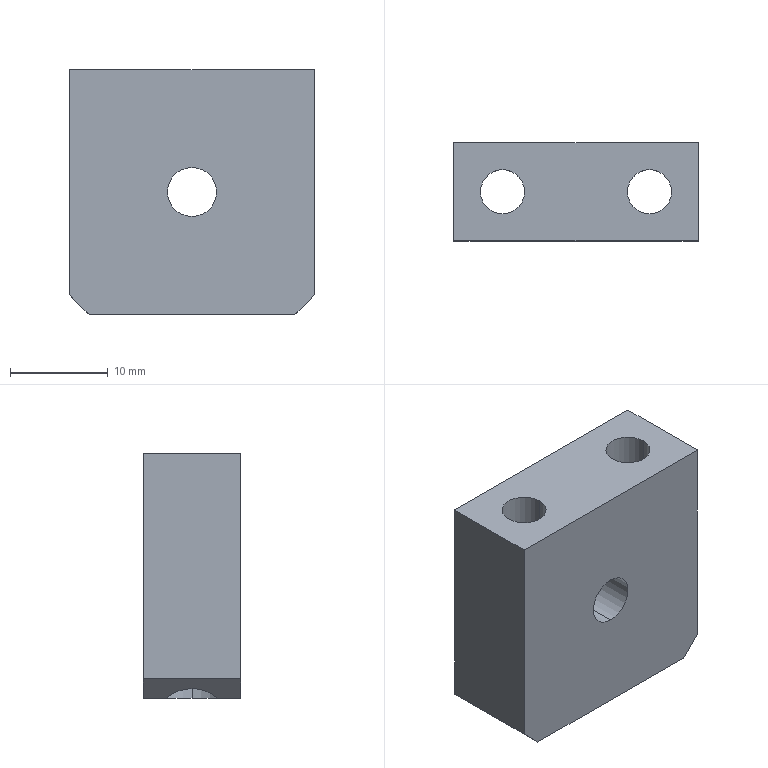Part | SolidWorks | features HoleWzd 2, Chamfer 1, Extrusion 1 | 1 solid | 20 faces | box 25 x 10 x 25 mm | volume 3874 mm3 | cylinder 10 | plane 10 | commonest cylinder face diameters 4.5 x4 8 x4 5 x2
STEP:
#1=CARTESIAN_POINT('',(11.5,5.,7.1));
#2=VERTEX_POINT('',#1);
#3=CARTESIAN_POINT('',(3.5,5.,7.1));
#4=VERTEX_POINT('',#3);
#5=CARTESIAN_POINT('',(7.5,5.,7.1));
#6=DIRECTION('',(0.,0.,-1.));
#7=DIRECTION('',(-1.,0.,0.));
#8=AXIS2_PLACEMENT_3D('',#5,#6,#7);
#9=CIRCLE('',#8,4.);
#10=EDGE_CURVE('',#2,#4,#9,.T.);
#11=ORIENTED_EDGE('',*,*,#10,.F.);
#12=CARTESIAN_POINT('',(11.5,5.,-11.5));
#13=VERTEX_POINT('',#12);
#14=CARTESIAN_POINT('',(11.5,5.,-12.5));
#15=DIRECTION('',(0.,0.,-1.));
#16=VECTOR('',#15,1000.);
#17=LINE('',#14,#16);
#18=EDGE_CURVE('',#2,#13,#17,.T.);
#19=ORIENTED_EDGE('',*,*,#18,.T.);
#20=CARTESIAN_POINT('',(10.5,2.354,-12.5));
#21=VERTEX_POINT('',#20);
#22=CARTESIAN_POINT('',(11.5,5.,-11.5));
#23=CARTESIAN_POINT('',(11.5,4.015,-11.5));
#24=CARTESIAN_POINT('',(11.152,3.093,-11.848));
#25=CARTESIAN_POINT('',(10.5,2.354,-12.5));
#26=(BOUNDED_CURVE()B_SPLINE_CURVE(3,(#22,#23,#24,#25),.UNSPECIFIED.,.F.,.F.)B_SPLINE_CURVE_WITH_KNOTS((4,4),(3.142,3.864),.UNSPECIFIED.)CURVE()GEOMETRIC_REPRESENTATION_ITEM()RATIONAL_B_SPLINE_CURVE((1.,0.9569,0.9569,1.))REPRESENTATION_ITEM(''));
#27=EDGE_CURVE('',#13,#21,#26,.T.);
#28=ORIENTED_EDGE('',*,*,#27,.T.);
#29=CARTESIAN_POINT('',(3.5,5.,-12.5));
#30=VERTEX_POINT('',#29);
#31=CARTESIAN_POINT('',(7.5,5.,-12.5));
#32=DIRECTION('',(0.,0.,-1.));
#33=DIRECTION('',(-1.,0.,0.));
#34=AXIS2_PLACEMENT_3D('',#31,#32,#33);
#35=CIRCLE('',#34,4.);
#36=EDGE_CURVE('',#21,#30,#35,.T.);
#37=ORIENTED_EDGE('',*,*,#36,.T.);
#38=CARTESIAN_POINT('',(3.5,5.,-12.5));
#39=DIRECTION('',(0.,0.,-1.));
#40=VECTOR('',#39,1000.);
#41=LINE('',#38,#40);
#42=EDGE_CURVE('',#4,#30,#41,.T.);
#43=ORIENTED_EDGE('',*,*,#42,.F.);
#44=EDGE_LOOP('',(#11,#19,#28,#37,#43));
#45=FACE_OUTER_BOUND('',#44,.T.);
#46=CARTESIAN_POINT('',(7.5,5.,-12.5));
#47=DIRECTION('',(0.,0.,-1.));
#48=DIRECTION('',(-1.,0.,0.));
#49=AXIS2_PLACEMENT_3D('',#46,#47,#48);
#50=CYLINDRICAL_SURFACE('',#49,4.);
#51=ADVANCED_FACE('',(#45),#50,.F.);
#52=CARTESIAN_POINT('',(9.75,5.,12.5));
#53=VERTEX_POINT('',#52);
#54=CARTESIAN_POINT('',(5.25,5.,12.5));
#55=VERTEX_POINT('',#54);
#56=CARTESIAN_POINT('',(7.5,5.,12.5));
#57=DIRECTION('',(0.,0.,-1.));
#58=DIRECTION('',(-1.,0.,0.));
#59=AXIS2_PLACEMENT_3D('',#56,#57,#58);
#60=CIRCLE('',#59,2.25);
#61=EDGE_CURVE('',#53,#55,#60,.T.);
#62=ORIENTED_EDGE('',*,*,#61,.F.);
#63=CARTESIAN_POINT('',(9.75,5.,7.1));
#64=VERTEX_POINT('',#63);
#65=CARTESIAN_POINT('',(9.75,5.,-12.5));
#66=DIRECTION('',(0.,0.,-1.));
#67=VECTOR('',#66,1000.);
#68=LINE('',#65,#67);
#69=EDGE_CURVE('',#53,#64,#68,.T.);
#70=ORIENTED_EDGE('',*,*,#69,.T.);
#71=CARTESIAN_POINT('',(5.25,5.,7.1));
#72=VERTEX_POINT('',#71);
#73=CARTESIAN_POINT('',(7.5,5.,7.1));
#74=DIRECTION('',(0.,0.,-1.));
#75=DIRECTION('',(-1.,0.,0.));
#76=AXIS2_PLACEMENT_3D('',#73,#74,#75);
#77=CIRCLE('',#76,2.25);
#78=EDGE_CURVE('',#64,#72,#77,.T.);
#79=ORIENTED_EDGE('',*,*,#78,.T.);
#80=CARTESIAN_POINT('',(5.25,5.,-12.5));
#81=DIRECTION('',(0.,0.,-1.));
#82=VECTOR('',#81,1000.);
#83=LINE('',#80,#82);
#84=EDGE_CURVE('',#55,#72,#83,.T.);
#85=ORIENTED_EDGE('',*,*,#84,.F.);
#86=EDGE_LOOP('',(#62,#70,#79,#85));
#87=FACE_OUTER_BOUND('',#86,.T.);
#88=CARTESIAN_POINT('',(7.5,5.,-12.5));
#89=DIRECTION('',(0.,0.,-1.));
#90=DIRECTION('',(-1.,0.,0.));
#91=AXIS2_PLACEMENT_3D('',#88,#89,#90);
#92=CYLINDRICAL_SURFACE('',#91,2.25);
#93=ADVANCED_FACE('',(#87),#92,.F.);
#94=CARTESIAN_POINT('',(-3.5,5.,7.1));
#95=VERTEX_POINT('',#94);
#96=CARTESIAN_POINT('',(-11.5,5.,7.1));
#97=VERTEX_POINT('',#96);
#98=CARTESIAN_POINT('',(-7.5,5.,7.1));
#99=DIRECTION('',(0.,0.,-1.));
#100=DIRECTION('',(-1.,0.,0.));
#101=AXIS2_PLACEMENT_3D('',#98,#99,#100);
#102=CIRCLE('',#101,4.);
#103=EDGE_CURVE('',#95,#97,#102,.T.);
#104=ORIENTED_EDGE('',*,*,#103,.F.);
#105=CARTESIAN_POINT('',(-3.5,5.,-12.5));
#106=VERTEX_POINT('',#105);
#107=CARTESIAN_POINT('',(-3.5,5.,-12.5));
#108=DIRECTION('',(0.,0.,-1.));
#109=VECTOR('',#108,1000.);
#110=LINE('',#107,#109);
#111=EDGE_CURVE('',#95,#106,#110,.T.);
#112=ORIENTED_EDGE('',*,*,#111,.T.);
#113=CARTESIAN_POINT('',(-10.5,2.354,-12.5));
#114=VERTEX_POINT('',#113);
#115=CARTESIAN_POINT('',(-7.5,5.,-12.5));
#116=DIRECTION('',(0.,0.,-1.));
#117=DIRECTION('',(-1.,0.,0.));
#118=AXIS2_PLACEMENT_3D('',#115,#116,#117);
#119=CIRCLE('',#118,4.);
#120=EDGE_CURVE('',#106,#114,#119,.T.);
#121=ORIENTED_EDGE('',*,*,#120,.T.);
#122=CARTESIAN_POINT('',(-11.5,5.,-11.5));
#123=VERTEX_POINT('',#122);
#124=CARTESIAN_POINT('',(-10.5,2.354,-12.5));
#125=CARTESIAN_POINT('',(-11.152,3.093,-11.848));
#126=CARTESIAN_POINT('',(-11.5,4.015,-11.5));
#127=CARTESIAN_POINT('',(-11.5,5.,-11.5));
#128=(BOUNDED_CURVE()B_SPLINE_CURVE(3,(#124,#125,#126,#127),.UNSPECIFIED.,.F.,.T.)B_SPLINE_CURVE_WITH_KNOTS((4,4),(2.419,3.142),.UNSPECIFIED.)CURVE()GEOMETRIC_REPRESENTATION_ITEM()RATIONAL_B_SPLINE_CURVE((1.,0.9569,0.9569,1.))REPRESENTATION_ITEM(''));
#129=EDGE_CURVE('',#114,#123,#128,.T.);
#130=ORIENTED_EDGE('',*,*,#129,.T.);
#131=CARTESIAN_POINT('',(-11.5,5.,-12.5));
#132=DIRECTION('',(0.,0.,-1.));
#133=VECTOR('',#132,1000.);
#134=LINE('',#131,#133);
#135=EDGE_CURVE('',#97,#123,#134,.T.);
#136=ORIENTED_EDGE('',*,*,#135,.F.);
#137=EDGE_LOOP('',(#104,#112,#121,#130,#136));
#138=FACE_OUTER_BOUND('',#137,.T.);
#139=CARTESIAN_POINT('',(-7.5,5.,-12.5));
#140=DIRECTION('',(0.,0.,-1.));
#141=DIRECTION('',(-1.,0.,0.));
#142=AXIS2_PLACEMENT_3D('',#139,#140,#141);
#143=CYLINDRICAL_SURFACE('',#142,4.);
#144=ADVANCED_FACE('',(#138),#143,.F.);
#145=CARTESIAN_POINT('',(-5.25,5.,12.5));
#146=VERTEX_POINT('',#145);
#147=CARTESIAN_POINT('',(-9.75,5.,12.5));
#148=VERTEX_POINT('',#147);
#149=CARTESIAN_POINT('',(-7.5,5.,12.5));
#150=DIRECTION('',(0.,0.,-1.));
#151=DIRECTION('',(-1.,0.,0.));
#152=AXIS2_PLACEMENT_3D('',#149,#150,#151);
#153=CIRCLE('',#152,2.25);
#154=EDGE_CURVE('',#146,#148,#153,.T.);
#155=ORIENTED_EDGE('',*,*,#154,.F.);
#156=CARTESIAN_POINT('',(-5.25,5.,7.1));
#157=VERTEX_POINT('',#156);
#158=CARTESIAN_POINT('',(-5.25,5.,-12.5));
#159=DIRECTION('',(0.,0.,-1.));
#160=VECTOR('',#159,1000.);
#161=LINE('',#158,#160);
#162=EDGE_CURVE('',#146,#157,#161,.T.);
#163=ORIENTED_EDGE('',*,*,#162,.T.);
#164=CARTESIAN_POINT('',(-9.75,5.,7.1));
#165=VERTEX_POINT('',#164);
#166=CARTESIAN_POINT('',(-7.5,5.,7.1));
#167=DIRECTION('',(0.,0.,-1.));
#168=DIRECTION('',(-1.,0.,0.));
#169=AXIS2_PLACEMENT_3D('',#166,#167,#168);
#170=CIRCLE('',#169,2.25);
#171=EDGE_CURVE('',#157,#165,#170,.T.);
#172=ORIENTED_EDGE('',*,*,#171,.T.);
#173=CARTESIAN_POINT('',(-9.75,5.,-12.5));
#174=DIRECTION('',(0.,0.,-1.));
#175=VECTOR('',#174,1000.);
#176=LINE('',#173,#175);
#177=EDGE_CURVE('',#148,#165,#176,.T.);
#178=ORIENTED_EDGE('',*,*,#177,.F.);
#179=EDGE_LOOP('',(#155,#163,#172,#178));
#180=FACE_OUTER_BOUND('',#179,.T.);
#181=CARTESIAN_POINT('',(-7.5,5.,-12.5));
#182=DIRECTION('',(0.,0.,-1.));
#183=DIRECTION('',(-1.,0.,0.));
#184=AXIS2_PLACEMENT_3D('',#181,#182,#183);
#185=CYLINDRICAL_SURFACE('',#184,2.25);
#186=ADVANCED_FACE('',(#180),#185,.F.);
#187=CARTESIAN_POINT('',(0.,10.,2.5));
#188=VERTEX_POINT('',#187);
#189=CARTESIAN_POINT('',(0.,10.,-2.5));
#190=VERTEX_POINT('',#189);
#191=CARTESIAN_POINT('',(0.,10.,0.));
#192=DIRECTION('',(0.,-1.,0.));
#193=DIRECTION('',(0.,0.,-1.));
#194=AXIS2_PLACEMENT_3D('',#191,#192,#193);
#195=CIRCLE('',#194,2.5);
#196=EDGE_CURVE('',#188,#190,#195,.T.);
#197=ORIENTED_EDGE('',*,*,#196,.F.);
#198=CARTESIAN_POINT('',(0.,0.,2.5));
#199=VERTEX_POINT('',#198);
#200=CARTESIAN_POINT('',(0.,0.,2.5));
#201=DIRECTION('',(0.,-1.,0.));
#202=VECTOR('',#201,1000.);
#203=LINE('',#200,#202);
#204=EDGE_CURVE('',#188,#199,#203,.T.);
#205=ORIENTED_EDGE('',*,*,#204,.T.);
#206=CARTESIAN_POINT('',(0.,0.,-2.5));
#207=VERTEX_POINT('',#206);
#208=CARTESIAN_POINT('',(0.,0.,0.));
#209=DIRECTION('',(0.,-1.,0.));
#210=DIRECTION('',(0.,0.,-1.));
#211=AXIS2_PLACEMENT_3D('',#208,#209,#210);
#212=CIRCLE('',#211,2.5);
#213=EDGE_CURVE('',#199,#207,#212,.T.);
#214=ORIENTED_EDGE('',*,*,#213,.T.);
#215=CARTESIAN_POINT('',(0.,0.,-2.5));
#216=DIRECTION('',(0.,-1.,0.));
#217=VECTOR('',#216,1000.);
#218=LINE('',#215,#217);
#219=EDGE_CURVE('',#190,#207,#218,.T.);
#220=ORIENTED_EDGE('',*,*,#219,.F.);
#221=EDGE_LOOP('',(#197,#205,#214,#220));
#222=FACE_OUTER_BOUND('',#221,.T.);
#223=CARTESIAN_POINT('',(0.,0.,0.));
#224=DIRECTION('',(0.,-1.,0.));
#225=DIRECTION('',(0.,0.,-1.));
#226=AXIS2_PLACEMENT_3D('',#223,#224,#225);
#227=CYLINDRICAL_SURFACE('',#226,2.5);
#228=ADVANCED_FACE('',(#222),#227,.F.);
#229=CARTESIAN_POINT('',(10.5,10.,-12.5));
#230=VERTEX_POINT('',#229);
#231=CARTESIAN_POINT('',(10.5,7.646,-12.5));
#232=VERTEX_POINT('',#231);
#233=CARTESIAN_POINT('',(10.5,10.,-12.5));
#234=DIRECTION('',(0.,-1.,0.));
#235=VECTOR('',#234,1000.);
#236=LINE('',#233,#235);
#237=EDGE_CURVE('',#230,#232,#236,.T.);
#238=ORIENTED_EDGE('',*,*,#237,.T.);
#239=CARTESIAN_POINT('',(7.5,5.,-12.5));
#240=DIRECTION('',(0.,0.,-1.));
#241=DIRECTION('',(-1.,0.,0.));
#242=AXIS2_PLACEMENT_3D('',#239,#240,#241);
#243=CIRCLE('',#242,4.);
#244=EDGE_CURVE('',#30,#232,#243,.T.);
#245=ORIENTED_EDGE('',*,*,#244,.F.);
#246=ORIENTED_EDGE('',*,*,#36,.F.);
#247=CARTESIAN_POINT('',(10.5,0.,-12.5));
#248=VERTEX_POINT('',#247);
#249=CARTESIAN_POINT('',(10.5,10.,-12.5));
#250=DIRECTION('',(0.,-1.,0.));
#251=VECTOR('',#250,1000.);
#252=LINE('',#249,#251);
#253=EDGE_CURVE('',#21,#248,#252,.T.);
#254=ORIENTED_EDGE('',*,*,#253,.T.);
#255=CARTESIAN_POINT('',(-10.5,0.,-12.5));
#256=VERTEX_POINT('',#255);
#257=CARTESIAN_POINT('',(-12.5,0.,-12.5));
#258=DIRECTION('',(-1.,0.,0.));
#259=VECTOR('',#258,1000.);
#260=LINE('',#257,#259);
#261=EDGE_CURVE('',#248,#256,#260,.T.);
#262=ORIENTED_EDGE('',*,*,#261,.T.);
#263=CARTESIAN_POINT('',(-10.5,10.,-12.5));
#264=DIRECTION('',(0.,1.,0.));
#265=VECTOR('',#264,1000.);
#266=LINE('',#263,#265);
#267=EDGE_CURVE('',#256,#114,#266,.T.);
#268=ORIENTED_EDGE('',*,*,#267,.T.);
#269=ORIENTED_EDGE('',*,*,#120,.F.);
#270=CARTESIAN_POINT('',(-10.5,7.646,-12.5));
#271=VERTEX_POINT('',#270);
#272=CARTESIAN_POINT('',(-7.5,5.,-12.5));
#273=DIRECTION('',(0.,0.,-1.));
#274=DIRECTION('',(-1.,0.,0.));
#275=AXIS2_PLACEMENT_3D('',#272,#273,#274);
#276=CIRCLE('',#275,4.);
#277=EDGE_CURVE('',#271,#106,#276,.T.);
#278=ORIENTED_EDGE('',*,*,#277,.F.);
#279=CARTESIAN_POINT('',(-10.5,10.,-12.5));
#280=VERTEX_POINT('',#279);
#281=CARTESIAN_POINT('',(-10.5,10.,-12.5));
#282=DIRECTION('',(0.,1.,0.));
#283=VECTOR('',#282,1000.);
#284=LINE('',#281,#283);
#285=EDGE_CURVE('',#271,#280,#284,.T.);
#286=ORIENTED_EDGE('',*,*,#285,.T.);
#287=CARTESIAN_POINT('',(-12.5,10.,-12.5));
#288=DIRECTION('',(-1.,0.,0.));
#289=VECTOR('',#288,1000.);
#290=LINE('',#287,#289);
#291=EDGE_CURVE('',#230,#280,#290,.T.);
#292=ORIENTED_EDGE('',*,*,#291,.F.);
#293=EDGE_LOOP('',(#238,#245,#246,#254,#262,#268,#269,#278,#286,#292));
#294=FACE_OUTER_BOUND('',#293,.T.);
#295=CARTESIAN_POINT('',(-12.5,10.,-12.5));
#296=DIRECTION('',(0.,0.,1.));
#297=DIRECTION('',(1.,0.,0.));
#298=AXIS2_PLACEMENT_3D('',#295,#296,#297);
#299=PLANE('',#298);
#300=ADVANCED_FACE('',(#294),#299,.F.);
#301=CARTESIAN_POINT('',(12.5,0.,12.5));
#302=VERTEX_POINT('',#301);
#303=CARTESIAN_POINT('',(12.5,0.,-10.5));
#304=VERTEX_POINT('',#303);
#305=CARTESIAN_POINT('',(12.5,0.,12.5));
#306=DIRECTION('',(0.,0.,-1.));
#307=VECTOR('',#306,1000.);
#308=LINE('',#305,#307);
#309=EDGE_CURVE('',#302,#304,#308,.T.);
#310=ORIENTED_EDGE('',*,*,#309,.T.);
#311=CARTESIAN_POINT('',(12.5,10.,-10.5));
#312=VERTEX_POINT('',#311);
#313=CARTESIAN_POINT('',(12.5,10.,-10.5));
#314=DIRECTION('',(0.,1.,0.));
#315=VECTOR('',#314,1000.);
#316=LINE('',#313,#315);
#317=EDGE_CURVE('',#304,#312,#316,.T.);
#318=ORIENTED_EDGE('',*,*,#317,.T.);
#319=CARTESIAN_POINT('',(12.5,10.,12.5));
#320=VERTEX_POINT('',#319);
#321=CARTESIAN_POINT('',(12.5,10.,12.5));
#322=DIRECTION('',(0.,0.,-1.));
#323=VECTOR('',#322,1000.);
#324=LINE('',#321,#323);
#325=EDGE_CURVE('',#320,#312,#324,.T.);
#326=ORIENTED_EDGE('',*,*,#325,.F.);
#327=CARTESIAN_POINT('',(12.5,10.,12.5));
#328=DIRECTION('',(0.,-1.,0.));
#329=VECTOR('',#328,1000.);
#330=LINE('',#327,#329);
#331=EDGE_CURVE('',#320,#302,#330,.T.);
#332=ORIENTED_EDGE('',*,*,#331,.T.);
#333=EDGE_LOOP('',(#310,#318,#326,#332));
#334=FACE_OUTER_BOUND('',#333,.T.);
#335=CARTESIAN_POINT('',(12.5,10.,12.5));
#336=DIRECTION('',(-1.,0.,0.));
#337=DIRECTION('',(0.,0.,1.));
#338=AXIS2_PLACEMENT_3D('',#335,#336,#337);
#339=PLANE('',#338);
#340=ADVANCED_FACE('',(#334),#339,.F.);
#341=CARTESIAN_POINT('',(-12.5,10.,-10.5));
#342=VERTEX_POINT('',#341);
#343=CARTESIAN_POINT('',(-12.5,10.,12.5));
#344=VERTEX_POINT('',#343);
#345=CARTESIAN_POINT('',(-12.5,10.,12.5));
#346=DIRECTION('',(0.,0.,1.));
#347=VECTOR('',#346,1000.);
#348=LINE('',#345,#347);
#349=EDGE_CURVE('',#342,#344,#348,.T.);
#350=ORIENTED_EDGE('',*,*,#349,.F.);
#351=CARTESIAN_POINT('',(-12.5,0.,-10.5));
#352=VERTEX_POINT('',#351);
#353=CARTESIAN_POINT('',(-12.5,10.,-10.5));
#354=DIRECTION('',(0.,-1.,0.));
#355=VECTOR('',#354,1000.);
#356=LINE('',#353,#355);
#357=EDGE_CURVE('',#342,#352,#356,.T.);
#358=ORIENTED_EDGE('',*,*,#357,.T.);
#359=CARTESIAN_POINT('',(-12.5,0.,12.5));
#360=VERTEX_POINT('',#359);
#361=CARTESIAN_POINT('',(-12.5,0.,12.5));
#362=DIRECTION('',(0.,0.,1.));
#363=VECTOR('',#362,1000.);
#364=LINE('',#361,#363);
#365=EDGE_CURVE('',#352,#360,#364,.T.);
#366=ORIENTED_EDGE('',*,*,#365,.T.);
#367=CARTESIAN_POINT('',(-12.5,10.,12.5));
#368=DIRECTION('',(0.,-1.,0.));
#369=VECTOR('',#368,1000.);
#370=LINE('',#367,#369);
#371=EDGE_CURVE('',#344,#360,#370,.T.);
#372=ORIENTED_EDGE('',*,*,#371,.F.);
#373=EDGE_LOOP('',(#350,#358,#366,#372));
#374=FACE_OUTER_BOUND('',#373,.T.);
#375=CARTESIAN_POINT('',(-12.5,10.,12.5));
#376=DIRECTION('',(1.,0.,0.));
#377=DIRECTION('',(0.,0.,-1.));
#378=AXIS2_PLACEMENT_3D('',#375,#376,#377);
#379=PLANE('',#378);
#380=ADVANCED_FACE('',(#374),#379,.F.);
#381=CARTESIAN_POINT('',(7.5,5.,12.5));
#382=DIRECTION('',(0.,0.,-1.));
#383=DIRECTION('',(-1.,0.,0.));
#384=AXIS2_PLACEMENT_3D('',#381,#382,#383);
#385=CIRCLE('',#384,2.25);
#386=EDGE_CURVE('',#55,#53,#385,.T.);
#387=ORIENTED_EDGE('',*,*,#386,.T.);
#388=ORIENTED_EDGE('',*,*,#61,.T.);
#389=EDGE_LOOP('',(#387,#388));
#390=FACE_BOUND('',#389,.T.);
#391=CARTESIAN_POINT('',(-7.5,5.,12.5));
#392=DIRECTION('',(0.,0.,-1.));
#393=DIRECTION('',(-1.,0.,0.));
#394=AXIS2_PLACEMENT_3D('',#391,#392,#393);
#395=CIRCLE('',#394,2.25);
#396=EDGE_CURVE('',#148,#146,#395,.T.);
#397=ORIENTED_EDGE('',*,*,#396,.T.);
#398=ORIENTED_EDGE('',*,*,#154,.T.);
#399=EDGE_LOOP('',(#397,#398));
#400=FACE_BOUND('',#399,.T.);
#401=CARTESIAN_POINT('',(-12.5,0.,12.5));
#402=DIRECTION('',(1.,0.,0.));
#403=VECTOR('',#402,1000.);
#404=LINE('',#401,#403);
#405=EDGE_CURVE('',#360,#302,#404,.T.);
#406=ORIENTED_EDGE('',*,*,#405,.T.);
#407=ORIENTED_EDGE('',*,*,#331,.F.);
#408=CARTESIAN_POINT('',(-12.5,10.,12.5));
#409=DIRECTION('',(1.,0.,0.));
#410=VECTOR('',#409,1000.);
#411=LINE('',#408,#410);
#412=EDGE_CURVE('',#344,#320,#411,.T.);
#413=ORIENTED_EDGE('',*,*,#412,.F.);
#414=ORIENTED_EDGE('',*,*,#371,.T.);
#415=EDGE_LOOP('',(#406,#407,#413,#414));
#416=FACE_OUTER_BOUND('',#415,.T.);
#417=CARTESIAN_POINT('',(-12.5,10.,12.5));
#418=DIRECTION('',(0.,0.,-1.));
#419=DIRECTION('',(-1.,0.,0.));
#420=AXIS2_PLACEMENT_3D('',#417,#418,#419);
#421=PLANE('',#420);
#422=ADVANCED_FACE('',(#390,#400,#416),#421,.F.);
#423=CARTESIAN_POINT('',(0.,10.,0.));
#424=DIRECTION('',(0.,-1.,0.));
#425=DIRECTION('',(0.,0.,-1.));
#426=AXIS2_PLACEMENT_3D('',#423,#424,#425);
#427=CIRCLE('',#426,2.5);
#428=EDGE_CURVE('',#190,#188,#427,.T.);
#429=ORIENTED_EDGE('',*,*,#428,.T.);
#430=ORIENTED_EDGE('',*,*,#196,.T.);
#431=EDGE_LOOP('',(#429,#430));
#432=FACE_BOUND('',#431,.T.);
#433=ORIENTED_EDGE('',*,*,#291,.T.);
#434=CARTESIAN_POINT('',(-12.5,10.,-10.5));
#435=DIRECTION('',(-0.7071,0.,0.7071));
#436=VECTOR('',#435,1000.);
#437=LINE('',#434,#436);
#438=EDGE_CURVE('',#280,#342,#437,.T.);
#439=ORIENTED_EDGE('',*,*,#438,.T.);
#440=ORIENTED_EDGE('',*,*,#349,.T.);
#441=ORIENTED_EDGE('',*,*,#412,.T.);
#442=ORIENTED_EDGE('',*,*,#325,.T.);
#443=CARTESIAN_POINT('',(10.5,10.,-12.5));
#444=DIRECTION('',(-0.7071,0.,-0.7071));
#445=VECTOR('',#444,1000.);
#446=LINE('',#443,#445);
#447=EDGE_CURVE('',#312,#230,#446,.T.);
#448=ORIENTED_EDGE('',*,*,#447,.T.);
#449=EDGE_LOOP('',(#433,#439,#440,#441,#442,#448));
#450=FACE_OUTER_BOUND('',#449,.T.);
#451=CARTESIAN_POINT('',(0.,10.,0.));
#452=DIRECTION('',(0.,-1.,0.));
#453=DIRECTION('',(0.,0.,-1.));
#454=AXIS2_PLACEMENT_3D('',#451,#452,#453);
#455=PLANE('',#454);
#456=ADVANCED_FACE('',(#432,#450),#455,.F.);
#457=CARTESIAN_POINT('',(0.,0.,0.));
#458=DIRECTION('',(0.,-1.,0.));
#459=DIRECTION('',(0.,0.,-1.));
#460=AXIS2_PLACEMENT_3D('',#457,#458,#459);
#461=CIRCLE('',#460,2.5);
#462=EDGE_CURVE('',#207,#199,#461,.T.);
#463=ORIENTED_EDGE('',*,*,#462,.F.);
#464=ORIENTED_EDGE('',*,*,#213,.F.);
#465=EDGE_LOOP('',(#463,#464));
#466=FACE_BOUND('',#465,.T.);
#467=ORIENTED_EDGE('',*,*,#365,.F.);
#468=CARTESIAN_POINT('',(-11.5,0.,-11.5));
#469=DIRECTION('',(0.7071,0.,-0.7071));
#470=VECTOR('',#469,1000.);
#471=LINE('',#468,#470);
#472=EDGE_CURVE('',#352,#256,#471,.T.);
#473=ORIENTED_EDGE('',*,*,#472,.T.);
#474=ORIENTED_EDGE('',*,*,#261,.F.);
#475=CARTESIAN_POINT('',(11.5,0.,-11.5));
#476=DIRECTION('',(0.7071,0.,0.7071));
#477=VECTOR('',#476,1000.);
#478=LINE('',#475,#477);
#479=EDGE_CURVE('',#248,#304,#478,.T.);
#480=ORIENTED_EDGE('',*,*,#479,.T.);
#481=ORIENTED_EDGE('',*,*,#309,.F.);
#482=ORIENTED_EDGE('',*,*,#405,.F.);
#483=EDGE_LOOP('',(#467,#473,#474,#480,#481,#482));
#484=FACE_OUTER_BOUND('',#483,.T.);
#485=CARTESIAN_POINT('',(0.,0.,0.));
#486=DIRECTION('',(0.,-1.,0.));
#487=DIRECTION('',(0.,0.,-1.));
#488=AXIS2_PLACEMENT_3D('',#485,#486,#487);
#489=PLANE('',#488);
#490=ADVANCED_FACE('',(#466,#484),#489,.T.);
#491=ORIENTED_EDGE('',*,*,#129,.F.);
#492=ORIENTED_EDGE('',*,*,#267,.F.);
#493=ORIENTED_EDGE('',*,*,#472,.F.);
#494=ORIENTED_EDGE('',*,*,#357,.F.);
#495=ORIENTED_EDGE('',*,*,#438,.F.);
#496=ORIENTED_EDGE('',*,*,#285,.F.);
#497=CARTESIAN_POINT('',(-11.5,5.,-11.5));
#498=CARTESIAN_POINT('',(-11.5,5.985,-11.5));
#499=CARTESIAN_POINT('',(-11.152,6.907,-11.848));
#500=CARTESIAN_POINT('',(-10.5,7.646,-12.5));
#501=(BOUNDED_CURVE()B_SPLINE_CURVE(3,(#497,#498,#499,#500),.UNSPECIFIED.,.F.,.F.)B_SPLINE_CURVE_WITH_KNOTS((4,4),(3.142,3.864),.UNSPECIFIED.)CURVE()GEOMETRIC_REPRESENTATION_ITEM()RATIONAL_B_SPLINE_CURVE((1.,0.9569,0.9569,1.))REPRESENTATION_ITEM(''));
#502=EDGE_CURVE('',#123,#271,#501,.T.);
#503=ORIENTED_EDGE('',*,*,#502,.F.);
#504=EDGE_LOOP('',(#491,#492,#493,#494,#495,#496,#503));
#505=FACE_OUTER_BOUND('',#504,.T.);
#506=CARTESIAN_POINT('',(-12.5,10.,-10.5));
#507=DIRECTION('',(0.7071,0.,0.7071));
#508=DIRECTION('',(0.,-1.,0.));
#509=AXIS2_PLACEMENT_3D('',#506,#507,#508);
#510=PLANE('',#509);
#511=ADVANCED_FACE('',(#505),#510,.F.);
#512=CARTESIAN_POINT('',(10.5,7.646,-12.5));
#513=CARTESIAN_POINT('',(11.152,6.907,-11.848));
#514=CARTESIAN_POINT('',(11.5,5.985,-11.5));
#515=CARTESIAN_POINT('',(11.5,5.,-11.5));
#516=(BOUNDED_CURVE()B_SPLINE_CURVE(3,(#512,#513,#514,#515),.UNSPECIFIED.,.F.,.F.)B_SPLINE_CURVE_WITH_KNOTS((4,4),(2.419,3.142),.UNSPECIFIED.)CURVE()GEOMETRIC_REPRESENTATION_ITEM()RATIONAL_B_SPLINE_CURVE((1.,0.9569,0.9569,1.))REPRESENTATION_ITEM(''));
#517=EDGE_CURVE('',#232,#13,#516,.T.);
#518=ORIENTED_EDGE('',*,*,#517,.F.);
#519=ORIENTED_EDGE('',*,*,#237,.F.);
#520=ORIENTED_EDGE('',*,*,#447,.F.);
#521=ORIENTED_EDGE('',*,*,#317,.F.);
#522=ORIENTED_EDGE('',*,*,#479,.F.);
#523=ORIENTED_EDGE('',*,*,#253,.F.);
#524=ORIENTED_EDGE('',*,*,#27,.F.);
#525=EDGE_LOOP('',(#518,#519,#520,#521,#522,#523,#524));
#526=FACE_OUTER_BOUND('',#525,.T.);
#527=CARTESIAN_POINT('',(10.5,10.,-12.5));
#528=DIRECTION('',(-0.7071,0.,0.7071));
#529=DIRECTION('',(0.,-1.,0.));
#530=AXIS2_PLACEMENT_3D('',#527,#528,#529);
#531=PLANE('',#530);
#532=ADVANCED_FACE('',(#526),#531,.F.);
#533=ORIENTED_EDGE('',*,*,#204,.F.);
#534=ORIENTED_EDGE('',*,*,#428,.F.);
#535=ORIENTED_EDGE('',*,*,#219,.T.);
#536=ORIENTED_EDGE('',*,*,#462,.T.);
#537=EDGE_LOOP('',(#533,#534,#535,#536));
#538=FACE_OUTER_BOUND('',#537,.T.);
#539=CARTESIAN_POINT('',(0.,0.,0.));
#540=DIRECTION('',(0.,-1.,0.));
#541=DIRECTION('',(0.,0.,-1.));
#542=AXIS2_PLACEMENT_3D('',#539,#540,#541);
#543=CYLINDRICAL_SURFACE('',#542,2.5);
#544=ADVANCED_FACE('',(#538),#543,.F.);
#545=ORIENTED_EDGE('',*,*,#162,.F.);
#546=ORIENTED_EDGE('',*,*,#396,.F.);
#547=ORIENTED_EDGE('',*,*,#177,.T.);
#548=CARTESIAN_POINT('',(-7.5,5.,7.1));
#549=DIRECTION('',(0.,0.,-1.));
#550=DIRECTION('',(-1.,0.,0.));
#551=AXIS2_PLACEMENT_3D('',#548,#549,#550);
#552=CIRCLE('',#551,2.25);
#553=EDGE_CURVE('',#165,#157,#552,.T.);
#554=ORIENTED_EDGE('',*,*,#553,.T.);
#555=EDGE_LOOP('',(#545,#546,#547,#554));
#556=FACE_OUTER_BOUND('',#555,.T.);
#557=CARTESIAN_POINT('',(-7.5,5.,-12.5));
#558=DIRECTION('',(0.,0.,-1.));
#559=DIRECTION('',(-1.,0.,0.));
#560=AXIS2_PLACEMENT_3D('',#557,#558,#559);
#561=CYLINDRICAL_SURFACE('',#560,2.25);
#562=ADVANCED_FACE('',(#556),#561,.F.);
#563=ORIENTED_EDGE('',*,*,#553,.F.);
#564=ORIENTED_EDGE('',*,*,#171,.F.);
#565=EDGE_LOOP('',(#563,#564));
#566=FACE_BOUND('',#565,.T.);
#567=CARTESIAN_POINT('',(-7.5,5.,7.1));
#568=DIRECTION('',(0.,0.,-1.));
#569=DIRECTION('',(-1.,0.,0.));
#570=AXIS2_PLACEMENT_3D('',#567,#568,#569);
#571=CIRCLE('',#570,4.);
#572=EDGE_CURVE('',#97,#95,#571,.T.);
#573=ORIENTED_EDGE('',*,*,#572,.T.);
#574=ORIENTED_EDGE('',*,*,#103,.T.);
#575=EDGE_LOOP('',(#573,#574));
#576=FACE_OUTER_BOUND('',#575,.T.);
#577=CARTESIAN_POINT('',(-5.25,5.,7.1));
#578=DIRECTION('',(0.,0.,1.));
#579=DIRECTION('',(1.,0.,0.));
#580=AXIS2_PLACEMENT_3D('',#577,#578,#579);
#581=PLANE('',#580);
#582=ADVANCED_FACE('',(#566,#576),#581,.F.);
#583=ORIENTED_EDGE('',*,*,#111,.F.);
#584=ORIENTED_EDGE('',*,*,#572,.F.);
#585=ORIENTED_EDGE('',*,*,#135,.T.);
#586=ORIENTED_EDGE('',*,*,#502,.T.);
#587=ORIENTED_EDGE('',*,*,#277,.T.);
#588=EDGE_LOOP('',(#583,#584,#585,#586,#587));
#589=FACE_OUTER_BOUND('',#588,.T.);
#590=CARTESIAN_POINT('',(-7.5,5.,-12.5));
#591=DIRECTION('',(0.,0.,-1.));
#592=DIRECTION('',(-1.,0.,0.));
#593=AXIS2_PLACEMENT_3D('',#590,#591,#592);
#594=CYLINDRICAL_SURFACE('',#593,4.);
#595=ADVANCED_FACE('',(#589),#594,.F.);
#596=ORIENTED_EDGE('',*,*,#69,.F.);
#597=ORIENTED_EDGE('',*,*,#386,.F.);
#598=ORIENTED_EDGE('',*,*,#84,.T.);
#599=CARTESIAN_POINT('',(7.5,5.,7.1));
#600=DIRECTION('',(0.,0.,-1.));
#601=DIRECTION('',(-1.,0.,0.));
#602=AXIS2_PLACEMENT_3D('',#599,#600,#601);
#603=CIRCLE('',#602,2.25);
#604=EDGE_CURVE('',#72,#64,#603,.T.);
#605=ORIENTED_EDGE('',*,*,#604,.T.);
#606=EDGE_LOOP('',(#596,#597,#598,#605));
#607=FACE_OUTER_BOUND('',#606,.T.);
#608=CARTESIAN_POINT('',(7.5,5.,-12.5));
#609=DIRECTION('',(0.,0.,-1.));
#610=DIRECTION('',(-1.,0.,0.));
#611=AXIS2_PLACEMENT_3D('',#608,#609,#610);
#612=CYLINDRICAL_SURFACE('',#611,2.25);
#613=ADVANCED_FACE('',(#607),#612,.F.);
#614=ORIENTED_EDGE('',*,*,#604,.F.);
#615=ORIENTED_EDGE('',*,*,#78,.F.);
#616=EDGE_LOOP('',(#614,#615));
#617=FACE_BOUND('',#616,.T.);
#618=CARTESIAN_POINT('',(7.5,5.,7.1));
#619=DIRECTION('',(0.,0.,-1.));
#620=DIRECTION('',(-1.,0.,0.));
#621=AXIS2_PLACEMENT_3D('',#618,#619,#620);
#622=CIRCLE('',#621,4.);
#623=EDGE_CURVE('',#4,#2,#622,.T.);
#624=ORIENTED_EDGE('',*,*,#623,.T.);
#625=ORIENTED_EDGE('',*,*,#10,.T.);
#626=EDGE_LOOP('',(#624,#625));
#627=FACE_OUTER_BOUND('',#626,.T.);
#628=CARTESIAN_POINT('',(9.75,5.,7.1));
#629=DIRECTION('',(0.,0.,1.));
#630=DIRECTION('',(1.,0.,0.));
#631=AXIS2_PLACEMENT_3D('',#628,#629,#630);
#632=PLANE('',#631);
#633=ADVANCED_FACE('',(#617,#627),#632,.F.);
#634=ORIENTED_EDGE('',*,*,#18,.F.);
#635=ORIENTED_EDGE('',*,*,#623,.F.);
#636=ORIENTED_EDGE('',*,*,#42,.T.);
#637=ORIENTED_EDGE('',*,*,#244,.T.);
#638=ORIENTED_EDGE('',*,*,#517,.T.);
#639=EDGE_LOOP('',(#634,#635,#636,#637,#638));
#640=FACE_OUTER_BOUND('',#639,.T.);
#641=CARTESIAN_POINT('',(7.5,5.,-12.5));
#642=DIRECTION('',(0.,0.,-1.));
#643=DIRECTION('',(-1.,0.,0.));
#644=AXIS2_PLACEMENT_3D('',#641,#642,#643);
#645=CYLINDRICAL_SURFACE('',#644,4.);
#646=ADVANCED_FACE('',(#640),#645,.F.);
#647=CLOSED_SHELL('',(#51,#93,#144,#186,#228,#300,#340,#380,#422,#456,#490,#511,#532,#544,#562,#582,#595,#613,#633,#646));
#648=MANIFOLD_SOLID_BREP('',#647);
#649=CARTESIAN_POINT('',(0.,0.,0.));
#650=DIRECTION('',(0.,0.,1.));
#651=DIRECTION('',(1.,0.,0.));
#652=AXIS2_PLACEMENT_3D('',#649,#650,#651);
#653=(LENGTH_UNIT()NAMED_UNIT(*)SI_UNIT(.MILLI.,.METRE.));
#654=UNCERTAINTY_MEASURE_WITH_UNIT(LENGTH_MEASURE(0.00001),#653,'','');
#655=(NAMED_UNIT(*)PLANE_ANGLE_UNIT()SI_UNIT($,.RADIAN.));
#656=(NAMED_UNIT(*)SI_UNIT($,.STERADIAN.)SOLID_ANGLE_UNIT());
#657=(GEOMETRIC_REPRESENTATION_CONTEXT(3)GLOBAL_UNCERTAINTY_ASSIGNED_CONTEXT((#654))GLOBAL_UNIT_ASSIGNED_CONTEXT((#653,#655,#656))REPRESENTATION_CONTEXT('',''));
#658=ADVANCED_BREP_SHAPE_REPRESENTATION('',(#648,#652),#657);